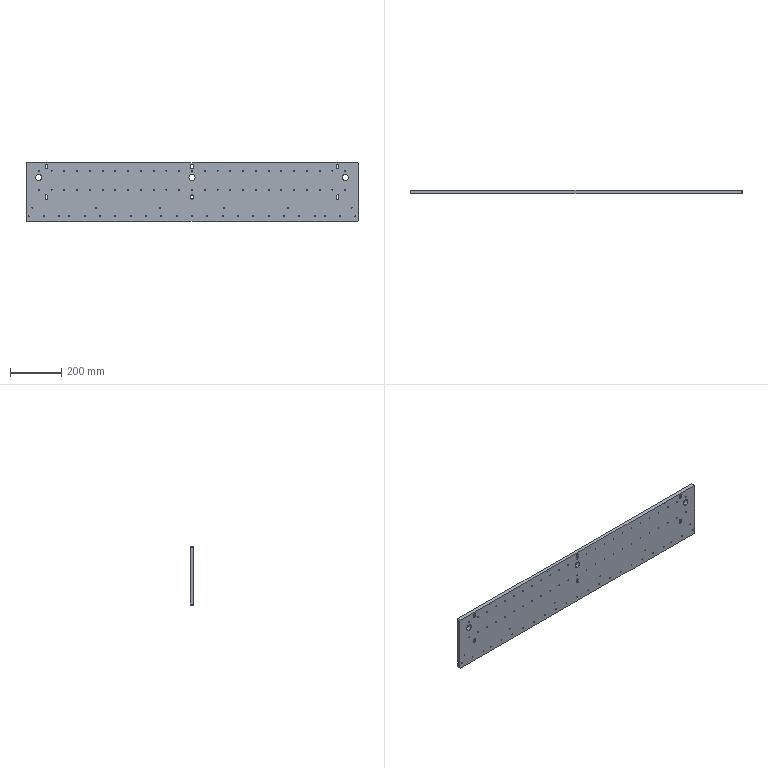Part | NX | features BREP 1 | 1 solid | 276 faces | box 1300 x 15 x 230 mm | volume 4372321 mm3 | cylinder 216 | plane 44 | cone 16 | commonest cylinder face diameters 4.2 x158 10 x18 15 x18 3.3 x16 25 x6